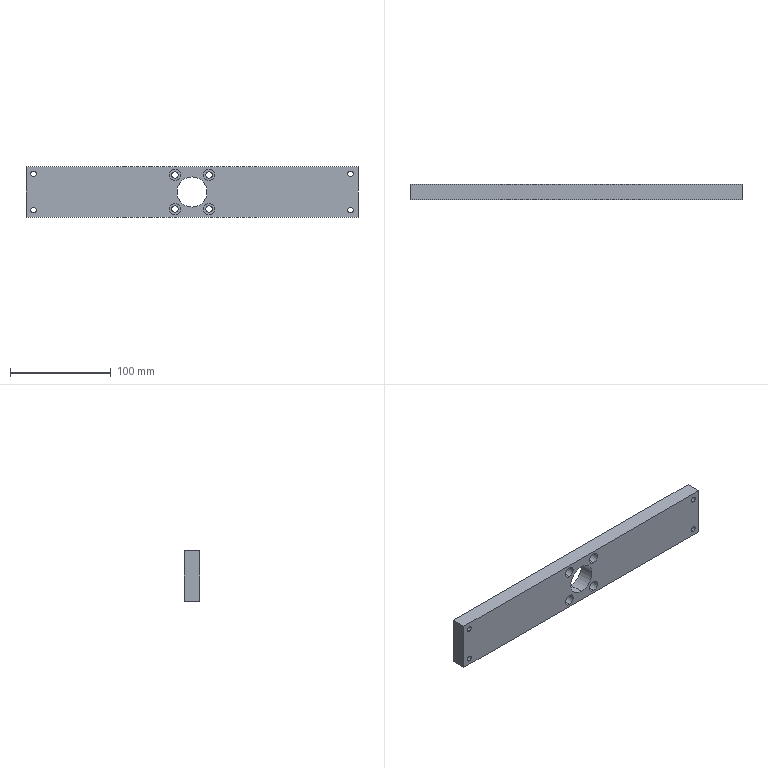Part | STEP file | A14-025 | 1 solid | 48 faces | box 330 x 15 x 50 mm | volume 229412 mm3 | cylinder 34 | plane 14 | commonest cylinder face diameters 5.5 x8 6.5 x8 9 x8 11 x8 30 x2